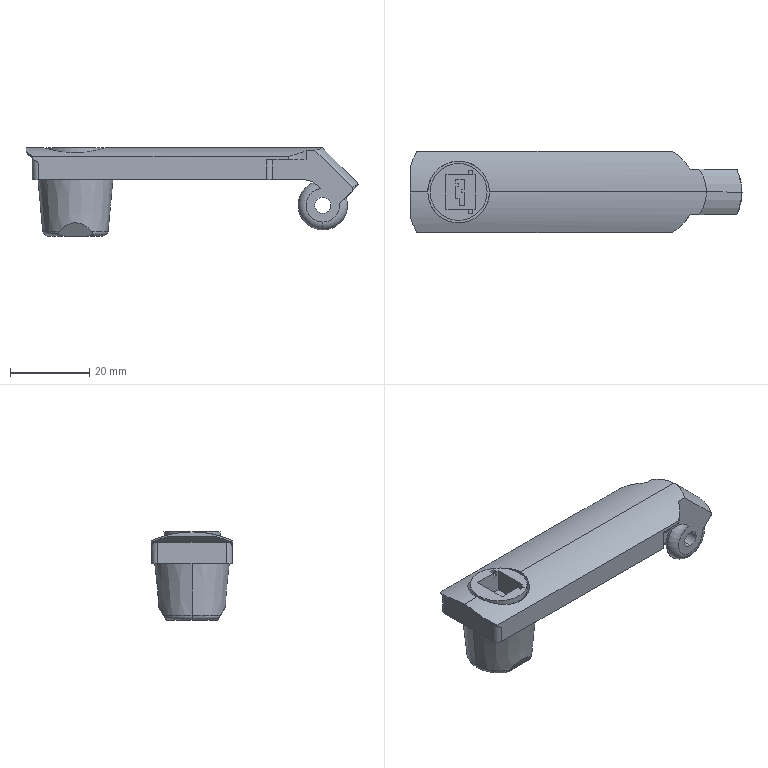Part | SolidWorks | features BaseBody 1 | 1 solid | 87 faces | box 83.993 x 20.5 x 22.3 mm | volume 13621 mm3 | plane 50 | cylinder 22 | torus 13 | cone 2 | commonest cylinder face diameters 4.1 x3 3 x2 3.2 x2 12.5 x2 14.4 x2 15.6 x2